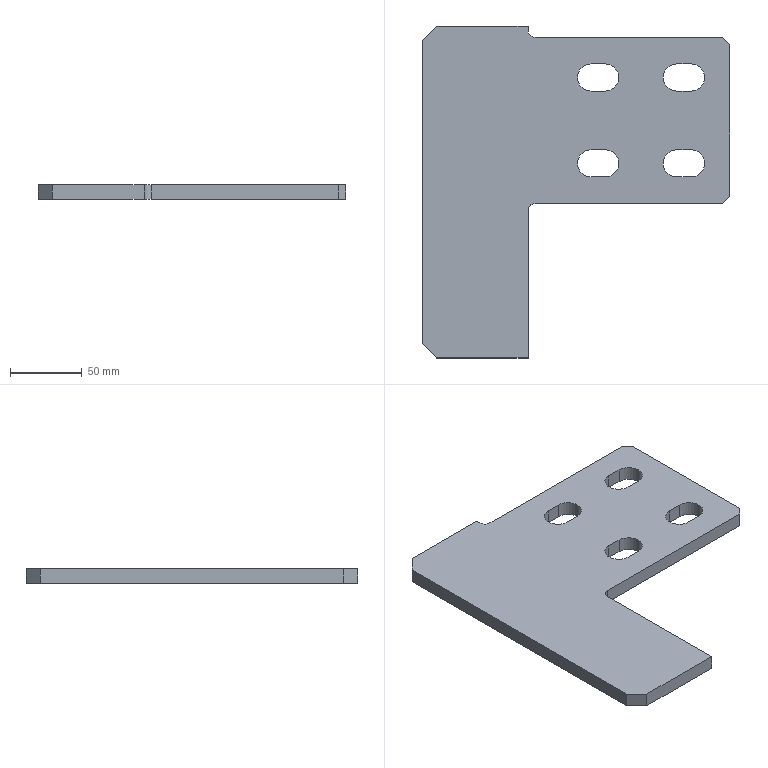Part | STEP file | 筋Plate-250×125-150-45度 | 1 solid | 36 faces | box 215 x 232 x 10 mm | volume 315156 mm3 | plane 22 | cylinder 14 | commonest cylinder face diameters 19 x12 10 x2